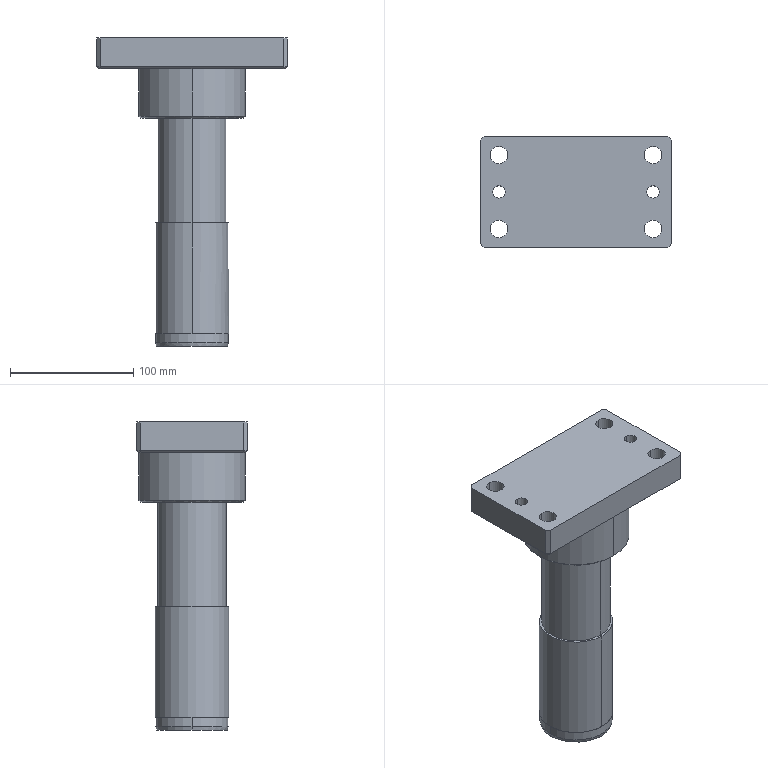Part | NX | features MI_MYKP_0166 2 | 1 solid | 203 faces | box 155 x 90 x 250 mm | volume 1040566 mm3 | plane 132 | cylinder 63 | cone 8 | commonest cylinder face diameters 14 x8 10 x4 50 x4 5.223 x3 6.232 x3 6.251 x3